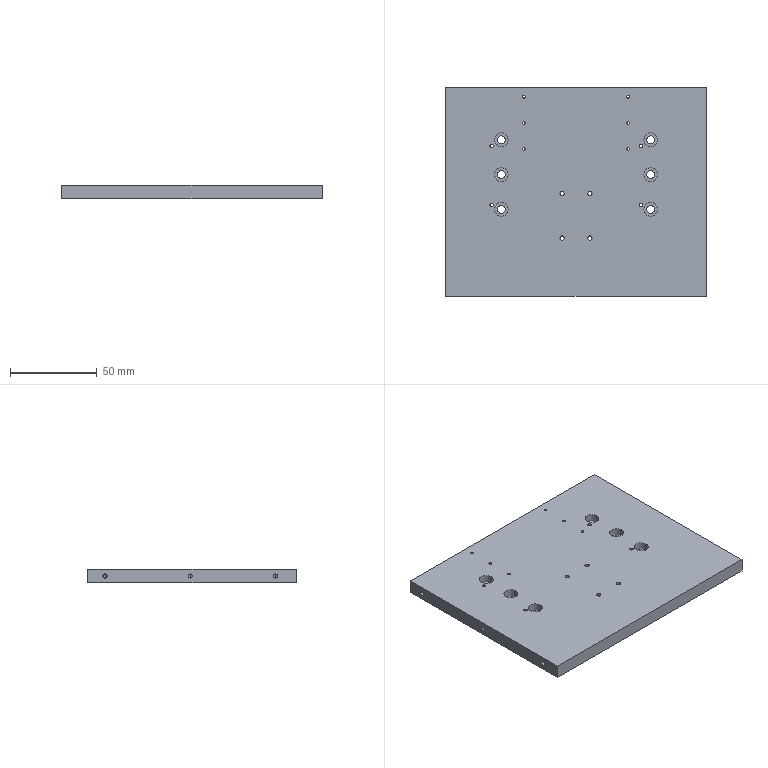Part | SolidWorks | features BaseBody 1 | 1 solid | 96 faces | box 150 x 120 x 8 mm | volume 141574 mm3 | cylinder 68 | cone 16 | plane 12 | commonest cylinder face diameters 2.459 x24 1.567 x12 4.5 x12 8 x12 2 x8